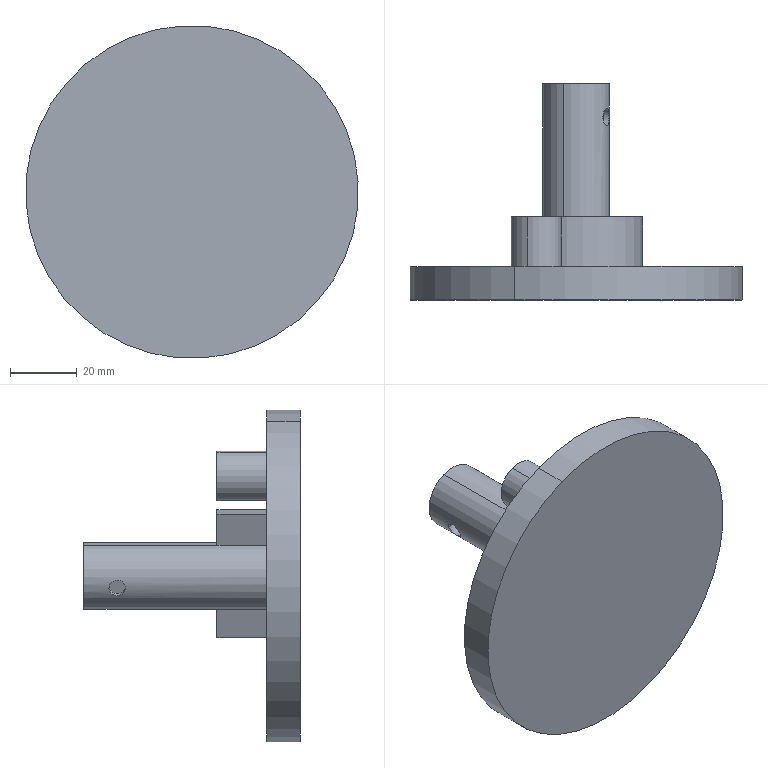Part | STEP file | Mirror 1 | 1 solid | 20 faces | box 100 x 65 x 100 mm | volume 105462 mm3 | cylinder 11 | plane 9 | commonest cylinder face diameters 5 x4 15 x2 20 x2 100 x2 40 x1
STEP:
#1=CARTESIAN_POINT('',(-1496.174,1582.764,2813.8));
#2=VERTEX_POINT('',#1);
#3=CARTESIAN_POINT('',(-1496.174,1587.764,2813.8));
#4=VERTEX_POINT('',#3);
#5=CARTESIAN_POINT('',(-1496.174,1585.264,2813.8));
#6=DIRECTION('',(0.9295,0.,0.3689));
#7=DIRECTION('',(0.,1.,0.));
#8=AXIS2_PLACEMENT_3D('',#5,#6,#7);
#9=CIRCLE('',#8,2.5);
#10=EDGE_CURVE('',#2,#4,#9,.T.);
#11=ORIENTED_EDGE('',*,*,#10,.T.);
#12=CARTESIAN_POINT('',(-1498.033,1587.764,2813.062));
#13=VERTEX_POINT('',#12);
#14=CARTESIAN_POINT('',(-1496.174,1587.764,2813.8));
#15=DIRECTION('',(0.9295,0.,0.3689));
#16=VECTOR('',#15,1000.);
#17=LINE('',#14,#16);
#18=EDGE_CURVE('',#13,#4,#17,.T.);
#19=ORIENTED_EDGE('',*,*,#18,.F.);
#20=CARTESIAN_POINT('',(-1498.033,1582.764,2813.062));
#21=VERTEX_POINT('',#20);
#22=CARTESIAN_POINT('',(-1498.033,1587.764,2813.062));
#23=CARTESIAN_POINT('',(-1497.972,1587.764,2812.908));
#24=CARTESIAN_POINT('',(-1497.908,1587.748,2812.758));
#25=CARTESIAN_POINT('',(-1497.775,1587.684,2812.466));
#26=CARTESIAN_POINT('',(-1497.706,1587.636,2812.322));
#27=CARTESIAN_POINT('',(-1497.567,1587.51,2812.052));
#28=CARTESIAN_POINT('',(-1497.498,1587.433,2811.925));
#29=CARTESIAN_POINT('',(-1497.363,1587.252,2811.687));
#30=CARTESIAN_POINT('',(-1497.296,1587.147,2811.576));
#31=CARTESIAN_POINT('',(-1497.111,1586.802,2811.279));
#32=CARTESIAN_POINT('',(-1497.004,1586.525,2811.121));
#33=CARTESIAN_POINT('',(-1496.894,1586.074,2810.963));
#34=CARTESIAN_POINT('',(-1496.865,1585.916,2810.923));
#35=CARTESIAN_POINT('',(-1496.826,1585.593,2810.869));
#36=CARTESIAN_POINT('',(-1496.816,1585.43,2810.855));
#37=CARTESIAN_POINT('',(-1496.816,1585.103,2810.855));
#38=CARTESIAN_POINT('',(-1496.826,1584.936,2810.869));
#39=CARTESIAN_POINT('',(-1496.864,1584.615,2810.922));
#40=CARTESIAN_POINT('',(-1496.893,1584.459,2810.962));
#41=CARTESIAN_POINT('',(-1497.004,1584.004,2811.121));
#42=CARTESIAN_POINT('',(-1497.11,1583.729,2811.276));
#43=CARTESIAN_POINT('',(-1497.296,1583.382,2811.576));
#44=CARTESIAN_POINT('',(-1497.361,1583.279,2811.685));
#45=CARTESIAN_POINT('',(-1497.496,1583.097,2811.922));
#46=CARTESIAN_POINT('',(-1497.567,1583.019,2812.051));
#47=CARTESIAN_POINT('',(-1497.705,1582.893,2812.321));
#48=CARTESIAN_POINT('',(-1497.773,1582.846,2812.462));
#49=CARTESIAN_POINT('',(-1497.907,1582.781,2812.755));
#50=CARTESIAN_POINT('',(-1497.972,1582.764,2812.908));
#51=CARTESIAN_POINT('',(-1498.033,1582.764,2813.062));
#52=B_SPLINE_CURVE_WITH_KNOTS('',3,(#22,#23,#24,#25,#26,#27,#28,#29,#30,#31,#32,#33,#34,#35,#36,#37,#38,#39,#40,#41,#42,#43,#44,#45,#46,#47,#48,#49,#50,#51),.UNSPECIFIED.,.F.,.F.,(4,2,2,2,2,2,2,2,2,2,2,2,2,2,4),(0.,0.0004903,0.0009806,0.001471,0.001961,0.002942,0.003432,0.003922,0.004413,0.004903,0.005884,0.006374,0.006864,0.007355,0.007845),.UNSPECIFIED.);
#53=EDGE_CURVE('',#13,#21,#52,.T.);
#54=ORIENTED_EDGE('',*,*,#53,.T.);
#55=CARTESIAN_POINT('',(-1496.174,1582.764,2813.8));
#56=DIRECTION('',(0.9295,0.,0.3689));
#57=VECTOR('',#56,1000.);
#58=LINE('',#55,#57);
#59=EDGE_CURVE('',#21,#2,#58,.T.);
#60=ORIENTED_EDGE('',*,*,#59,.T.);
#61=EDGE_LOOP('',(#11,#19,#54,#60));
#62=FACE_OUTER_BOUND('',#61,.T.);
#63=CARTESIAN_POINT('',(-1496.174,1585.264,2813.8));
#64=DIRECTION('',(-0.9295,0.,-0.3689));
#65=DIRECTION('',(0.,1.,0.));
#66=AXIS2_PLACEMENT_3D('',#63,#64,#65);
#67=CYLINDRICAL_SURFACE('',#66,2.5);
#68=ADVANCED_FACE('',(#62),#67,.F.);
#69=CARTESIAN_POINT('',(-1481.302,1582.764,2819.702));
#70=VERTEX_POINT('',#69);
#71=CARTESIAN_POINT('',(-1481.302,1587.764,2819.702));
#72=VERTEX_POINT('',#71);
#73=CARTESIAN_POINT('',(-1481.302,1585.264,2819.702));
#74=DIRECTION('',(0.9295,0.,0.3689));
#75=DIRECTION('',(0.,1.,0.));
#76=AXIS2_PLACEMENT_3D('',#73,#74,#75);
#77=CIRCLE('',#76,2.5);
#78=EDGE_CURVE('',#70,#72,#77,.T.);
#79=ORIENTED_EDGE('',*,*,#78,.F.);
#80=CARTESIAN_POINT('',(-1479.444,1582.764,2820.44));
#81=VERTEX_POINT('',#80);
#82=CARTESIAN_POINT('',(-1481.302,1582.764,2819.702));
#83=DIRECTION('',(0.9295,0.,0.3689));
#84=VECTOR('',#83,1000.);
#85=LINE('',#82,#84);
#86=EDGE_CURVE('',#70,#81,#85,.T.);
#87=ORIENTED_EDGE('',*,*,#86,.T.);
#88=CARTESIAN_POINT('',(-1479.444,1587.764,2820.44));
#89=VERTEX_POINT('',#88);
#90=CARTESIAN_POINT('',(-1479.444,1587.764,2820.44));
#91=CARTESIAN_POINT('',(-1479.382,1587.764,2820.285));
#92=CARTESIAN_POINT('',(-1479.326,1587.748,2820.132));
#93=CARTESIAN_POINT('',(-1479.222,1587.684,2819.829));
#94=CARTESIAN_POINT('',(-1479.175,1587.636,2819.677));
#95=CARTESIAN_POINT('',(-1479.09,1587.51,2819.385));
#96=CARTESIAN_POINT('',(-1479.053,1587.433,2819.245));
#97=CARTESIAN_POINT('',(-1478.989,1587.252,2818.979));
#98=CARTESIAN_POINT('',(-1478.961,1587.147,2818.853));
#99=CARTESIAN_POINT('',(-1478.891,1586.802,2818.51));
#100=CARTESIAN_POINT('',(-1478.862,1586.525,2818.321));
#101=CARTESIAN_POINT('',(-1478.834,1586.074,2818.131));
#102=CARTESIAN_POINT('',(-1478.827,1585.916,2818.081));
#103=CARTESIAN_POINT('',(-1478.819,1585.593,2818.015));
#104=CARTESIAN_POINT('',(-1478.816,1585.43,2817.999));
#105=CARTESIAN_POINT('',(-1478.816,1585.103,2817.999));
#106=CARTESIAN_POINT('',(-1478.819,1584.936,2818.015));
#107=CARTESIAN_POINT('',(-1478.827,1584.615,2818.081));
#108=CARTESIAN_POINT('',(-1478.834,1584.459,2818.129));
#109=CARTESIAN_POINT('',(-1478.861,1584.004,2818.321));
#110=CARTESIAN_POINT('',(-1478.891,1583.729,2818.507));
#111=CARTESIAN_POINT('',(-1478.961,1583.382,2818.853));
#112=CARTESIAN_POINT('',(-1478.988,1583.279,2818.977));
#113=CARTESIAN_POINT('',(-1479.053,1583.097,2819.242));
#114=CARTESIAN_POINT('',(-1479.09,1583.019,2819.384));
#115=CARTESIAN_POINT('',(-1479.174,1582.893,2819.676));
#116=CARTESIAN_POINT('',(-1479.221,1582.846,2819.825));
#117=CARTESIAN_POINT('',(-1479.325,1582.781,2820.13));
#118=CARTESIAN_POINT('',(-1479.382,1582.764,2820.285));
#119=CARTESIAN_POINT('',(-1479.444,1582.764,2820.44));
#120=B_SPLINE_CURVE_WITH_KNOTS('',3,(#90,#91,#92,#93,#94,#95,#96,#97,#98,#99,#100,#101,#102,#103,#104,#105,#106,#107,#108,#109,#110,#111,#112,#113,#114,#115,#116,#117,#118,#119),.UNSPECIFIED.,.F.,.F.,(4,2,2,2,2,2,2,2,2,2,2,2,2,2,4),(0.,0.0004903,0.0009806,0.001471,0.001961,0.002942,0.003432,0.003922,0.004413,0.004903,0.005884,0.006374,0.006864,0.007355,0.007845),.UNSPECIFIED.);
#121=EDGE_CURVE('',#89,#81,#120,.T.);
#122=ORIENTED_EDGE('',*,*,#121,.F.);
#123=CARTESIAN_POINT('',(-1481.302,1587.764,2819.702));
#124=DIRECTION('',(0.9295,0.,0.3689));
#125=VECTOR('',#124,1000.);
#126=LINE('',#123,#125);
#127=EDGE_CURVE('',#72,#89,#126,.T.);
#128=ORIENTED_EDGE('',*,*,#127,.F.);
#129=EDGE_LOOP('',(#79,#87,#122,#128));
#130=FACE_OUTER_BOUND('',#129,.T.);
#131=CARTESIAN_POINT('',(-1481.302,1585.264,2819.702));
#132=DIRECTION('',(0.9295,0.,0.3689));
#133=DIRECTION('',(0.,-1.,0.));
#134=AXIS2_PLACEMENT_3D('',#131,#132,#133);
#135=CYLINDRICAL_SURFACE('',#134,2.5);
#136=ADVANCED_FACE('',(#130),#135,.F.);
#137=CARTESIAN_POINT('',(-1503.438,1555.264,2853.79));
#138=VERTEX_POINT('',#137);
#139=CARTESIAN_POINT('',(-1497.905,1555.264,2839.848));
#140=VERTEX_POINT('',#139);
#141=CARTESIAN_POINT('',(-1500.672,1555.264,2846.819));
#142=DIRECTION('',(0.,1.,0.));
#143=DIRECTION('',(-0.3689,0.,0.9295));
#144=AXIS2_PLACEMENT_3D('',#141,#142,#143);
#145=CIRCLE('',#144,7.5);
#146=EDGE_CURVE('',#138,#140,#145,.T.);
#147=ORIENTED_EDGE('',*,*,#146,.F.);
#148=CARTESIAN_POINT('',(-1503.438,1540.264,2853.79));
#149=VERTEX_POINT('',#148);
#150=CARTESIAN_POINT('',(-1503.438,1555.264,2853.79));
#151=DIRECTION('',(0.,1.,0.));
#152=VECTOR('',#151,1000.);
#153=LINE('',#150,#152);
#154=EDGE_CURVE('',#149,#138,#153,.T.);
#155=ORIENTED_EDGE('',*,*,#154,.F.);
#156=CARTESIAN_POINT('',(-1497.905,1540.264,2839.848));
#157=VERTEX_POINT('',#156);
#158=CARTESIAN_POINT('',(-1500.672,1540.264,2846.819));
#159=DIRECTION('',(0.,1.,0.));
#160=DIRECTION('',(-0.3689,0.,0.9295));
#161=AXIS2_PLACEMENT_3D('',#158,#159,#160);
#162=CIRCLE('',#161,7.5);
#163=EDGE_CURVE('',#149,#157,#162,.T.);
#164=ORIENTED_EDGE('',*,*,#163,.T.);
#165=CARTESIAN_POINT('',(-1497.905,1555.264,2839.848));
#166=DIRECTION('',(0.,1.,0.));
#167=VECTOR('',#166,1000.);
#168=LINE('',#165,#167);
#169=EDGE_CURVE('',#157,#140,#168,.T.);
#170=ORIENTED_EDGE('',*,*,#169,.T.);
#171=EDGE_LOOP('',(#147,#155,#164,#170));
#172=FACE_OUTER_BOUND('',#171,.T.);
#173=CARTESIAN_POINT('',(-1500.672,1555.264,2846.819));
#174=DIRECTION('',(0.,-1.,0.));
#175=DIRECTION('',(-0.3689,0.,0.9295));
#176=AXIS2_PLACEMENT_3D('',#173,#174,#175);
#177=CYLINDRICAL_SURFACE('',#176,7.5);
#178=ADVANCED_FACE('',(#172),#177,.T.);
#179=CARTESIAN_POINT('',(-1507.183,1540.264,2863.224));
#180=VERTEX_POINT('',#179);
#181=CARTESIAN_POINT('',(-1470.294,1540.264,2770.277));
#182=VERTEX_POINT('',#181);
#183=CARTESIAN_POINT('',(-1488.738,1540.264,2816.751));
#184=DIRECTION('',(0.,1.,0.));
#185=DIRECTION('',(-0.3689,0.,0.9295));
#186=AXIS2_PLACEMENT_3D('',#183,#184,#185);
#187=CIRCLE('',#186,50.);
#188=EDGE_CURVE('',#180,#182,#187,.T.);
#189=ORIENTED_EDGE('',*,*,#188,.F.);
#190=CARTESIAN_POINT('',(-1507.183,1530.264,2863.224));
#191=VERTEX_POINT('',#190);
#192=CARTESIAN_POINT('',(-1507.183,1540.264,2863.224));
#193=DIRECTION('',(0.,1.,0.));
#194=VECTOR('',#193,1000.);
#195=LINE('',#192,#194);
#196=EDGE_CURVE('',#191,#180,#195,.T.);
#197=ORIENTED_EDGE('',*,*,#196,.F.);
#198=CARTESIAN_POINT('',(-1470.294,1530.264,2770.277));
#199=VERTEX_POINT('',#198);
#200=CARTESIAN_POINT('',(-1488.738,1530.264,2816.751));
#201=DIRECTION('',(0.,1.,0.));
#202=DIRECTION('',(-0.3689,0.,0.9295));
#203=AXIS2_PLACEMENT_3D('',#200,#201,#202);
#204=CIRCLE('',#203,50.);
#205=EDGE_CURVE('',#191,#199,#204,.T.);
#206=ORIENTED_EDGE('',*,*,#205,.T.);
#207=CARTESIAN_POINT('',(-1470.294,1540.264,2770.277));
#208=DIRECTION('',(0.,1.,0.));
#209=VECTOR('',#208,1000.);
#210=LINE('',#207,#209);
#211=EDGE_CURVE('',#199,#182,#210,.T.);
#212=ORIENTED_EDGE('',*,*,#211,.T.);
#213=EDGE_LOOP('',(#189,#197,#206,#212));
#214=FACE_OUTER_BOUND('',#213,.T.);
#215=CARTESIAN_POINT('',(-1488.738,1540.264,2816.751));
#216=DIRECTION('',(0.,-1.,0.));
#217=DIRECTION('',(-0.3689,0.,0.9295));
#218=AXIS2_PLACEMENT_3D('',#215,#216,#217);
#219=CYLINDRICAL_SURFACE('',#218,50.);
#220=ADVANCED_FACE('',(#214),#219,.T.);
#221=ORIENTED_EDGE('',*,*,#121,.T.);
#222=CARTESIAN_POINT('',(-1479.444,1582.764,2820.44));
#223=CARTESIAN_POINT('',(-1479.505,1582.764,2820.594));
#224=CARTESIAN_POINT('',(-1479.569,1582.781,2820.744));
#225=CARTESIAN_POINT('',(-1479.701,1582.845,2821.036));
#226=CARTESIAN_POINT('',(-1479.771,1582.893,2821.179));
#227=CARTESIAN_POINT('',(-1479.91,1583.019,2821.45));
#228=CARTESIAN_POINT('',(-1479.979,1583.095,2821.576));
#229=CARTESIAN_POINT('',(-1480.114,1583.277,2821.814));
#230=CARTESIAN_POINT('',(-1480.181,1583.382,2821.926));
#231=CARTESIAN_POINT('',(-1480.365,1583.726,2822.223));
#232=CARTESIAN_POINT('',(-1480.472,1584.004,2822.38));
#233=CARTESIAN_POINT('',(-1480.583,1584.455,2822.538));
#234=CARTESIAN_POINT('',(-1480.612,1584.613,2822.579));
#235=CARTESIAN_POINT('',(-1480.651,1584.936,2822.633));
#236=CARTESIAN_POINT('',(-1480.661,1585.098,2822.646));
#237=CARTESIAN_POINT('',(-1480.661,1585.426,2822.646));
#238=CARTESIAN_POINT('',(-1480.651,1585.592,2822.633));
#239=CARTESIAN_POINT('',(-1480.612,1585.913,2822.579));
#240=CARTESIAN_POINT('',(-1480.584,1586.069,2822.54));
#241=CARTESIAN_POINT('',(-1480.473,1586.525,2822.381));
#242=CARTESIAN_POINT('',(-1480.367,1586.8,2822.225));
#243=CARTESIAN_POINT('',(-1480.18,1587.147,2821.925));
#244=CARTESIAN_POINT('',(-1480.115,1587.25,2821.816));
#245=CARTESIAN_POINT('',(-1479.98,1587.431,2821.579));
#246=CARTESIAN_POINT('',(-1479.91,1587.51,2821.45));
#247=CARTESIAN_POINT('',(-1479.772,1587.635,2821.18));
#248=CARTESIAN_POINT('',(-1479.703,1587.683,2821.04));
#249=CARTESIAN_POINT('',(-1479.57,1587.748,2820.746));
#250=CARTESIAN_POINT('',(-1479.505,1587.764,2820.594));
#251=CARTESIAN_POINT('',(-1479.444,1587.764,2820.44));
#252=B_SPLINE_CURVE_WITH_KNOTS('',3,(#222,#223,#224,#225,#226,#227,#228,#229,#230,#231,#232,#233,#234,#235,#236,#237,#238,#239,#240,#241,#242,#243,#244,#245,#246,#247,#248,#249,#250,#251),.UNSPECIFIED.,.F.,.F.,(4,2,2,2,2,2,2,2,2,2,2,2,2,2,4),(0.,0.0004903,0.0009806,0.001471,0.001961,0.002942,0.003432,0.003922,0.004413,0.004903,0.005884,0.006374,0.006864,0.007355,0.007845),.UNSPECIFIED.);
#253=EDGE_CURVE('',#81,#89,#252,.T.);
#254=ORIENTED_EDGE('',*,*,#253,.T.);
#255=EDGE_LOOP('',(#221,#254));
#256=FACE_BOUND('',#255,.T.);
#257=CARTESIAN_POINT('',(-1492.427,1595.264,2826.045));
#258=VERTEX_POINT('',#257);
#259=CARTESIAN_POINT('',(-1485.049,1595.264,2807.456));
#260=VERTEX_POINT('',#259);
#261=CARTESIAN_POINT('',(-1488.738,1595.264,2816.751));
#262=DIRECTION('',(0.,1.,0.));
#263=DIRECTION('',(-0.3689,0.,0.9295));
#264=AXIS2_PLACEMENT_3D('',#261,#262,#263);
#265=CIRCLE('',#264,10.);
#266=EDGE_CURVE('',#258,#260,#265,.T.);
#267=ORIENTED_EDGE('',*,*,#266,.F.);
#268=CARTESIAN_POINT('',(-1492.427,1555.264,2826.045));
#269=VERTEX_POINT('',#268);
#270=CARTESIAN_POINT('',(-1492.427,1595.264,2826.045));
#271=DIRECTION('',(0.,1.,0.));
#272=VECTOR('',#271,1000.);
#273=LINE('',#270,#272);
#274=EDGE_CURVE('',#269,#258,#273,.T.);
#275=ORIENTED_EDGE('',*,*,#274,.F.);
#276=CARTESIAN_POINT('',(-1485.049,1555.264,2807.456));
#277=VERTEX_POINT('',#276);
#278=CARTESIAN_POINT('',(-1488.738,1555.264,2816.751));
#279=DIRECTION('',(0.,1.,0.));
#280=DIRECTION('',(-0.3689,0.,0.9295));
#281=AXIS2_PLACEMENT_3D('',#278,#279,#280);
#282=CIRCLE('',#281,10.);
#283=EDGE_CURVE('',#269,#277,#282,.T.);
#284=ORIENTED_EDGE('',*,*,#283,.T.);
#285=CARTESIAN_POINT('',(-1485.049,1595.264,2807.456));
#286=DIRECTION('',(0.,1.,0.));
#287=VECTOR('',#286,1000.);
#288=LINE('',#285,#287);
#289=EDGE_CURVE('',#277,#260,#288,.T.);
#290=ORIENTED_EDGE('',*,*,#289,.T.);
#291=EDGE_LOOP('',(#267,#275,#284,#290));
#292=FACE_OUTER_BOUND('',#291,.T.);
#293=CARTESIAN_POINT('',(-1488.738,1595.264,2816.751));
#294=DIRECTION('',(0.,-1.,0.));
#295=DIRECTION('',(-0.3689,0.,0.9295));
#296=AXIS2_PLACEMENT_3D('',#293,#294,#295);
#297=CYLINDRICAL_SURFACE('',#296,10.);
#298=ADVANCED_FACE('',(#256,#292),#297,.T.);
#299=ORIENTED_EDGE('',*,*,#274,.T.);
#300=CARTESIAN_POINT('',(-1488.738,1595.264,2816.751));
#301=DIRECTION('',(0.,1.,0.));
#302=DIRECTION('',(-0.3689,0.,0.9295));
#303=AXIS2_PLACEMENT_3D('',#300,#301,#302);
#304=CIRCLE('',#303,10.);
#305=EDGE_CURVE('',#260,#258,#304,.T.);
#306=ORIENTED_EDGE('',*,*,#305,.F.);
#307=ORIENTED_EDGE('',*,*,#289,.F.);
#308=CARTESIAN_POINT('',(-1485.049,1540.264,2807.456));
#309=VERTEX_POINT('',#308);
#310=CARTESIAN_POINT('',(-1485.049,1511.98,2807.456));
#311=DIRECTION('',(0.,-1.,0.));
#312=VECTOR('',#311,1000.);
#313=LINE('',#310,#312);
#314=EDGE_CURVE('',#277,#309,#313,.T.);
#315=ORIENTED_EDGE('',*,*,#314,.T.);
#316=CARTESIAN_POINT('',(-1492.427,1540.264,2826.045));
#317=VERTEX_POINT('',#316);
#318=CARTESIAN_POINT('',(-1488.738,1540.264,2816.751));
#319=DIRECTION('',(0.,1.,0.));
#320=DIRECTION('',(-0.3689,0.,0.9295));
#321=AXIS2_PLACEMENT_3D('',#318,#319,#320);
#322=CIRCLE('',#321,10.);
#323=EDGE_CURVE('',#309,#317,#322,.T.);
#324=ORIENTED_EDGE('',*,*,#323,.T.);
#325=CARTESIAN_POINT('',(-1492.427,1511.98,2826.045));
#326=DIRECTION('',(0.,1.,0.));
#327=VECTOR('',#326,1000.);
#328=LINE('',#325,#327);
#329=EDGE_CURVE('',#317,#269,#328,.T.);
#330=ORIENTED_EDGE('',*,*,#329,.T.);
#331=EDGE_LOOP('',(#299,#306,#307,#315,#324,#330));
#332=FACE_OUTER_BOUND('',#331,.T.);
#333=CARTESIAN_POINT('',(-1498.033,1582.764,2813.062));
#334=CARTESIAN_POINT('',(-1498.094,1582.764,2813.216));
#335=CARTESIAN_POINT('',(-1498.15,1582.781,2813.369));
#336=CARTESIAN_POINT('',(-1498.254,1582.845,2813.672));
#337=CARTESIAN_POINT('',(-1498.302,1582.893,2813.825));
#338=CARTESIAN_POINT('',(-1498.386,1583.019,2814.117));
#339=CARTESIAN_POINT('',(-1498.423,1583.095,2814.256));
#340=CARTESIAN_POINT('',(-1498.488,1583.277,2814.522));
#341=CARTESIAN_POINT('',(-1498.516,1583.382,2814.649));
#342=CARTESIAN_POINT('',(-1498.585,1583.726,2814.992));
#343=CARTESIAN_POINT('',(-1498.615,1584.004,2815.18));
#344=CARTESIAN_POINT('',(-1498.643,1584.455,2815.371));
#345=CARTESIAN_POINT('',(-1498.649,1584.613,2815.42));
#346=CARTESIAN_POINT('',(-1498.658,1584.936,2815.486));
#347=CARTESIAN_POINT('',(-1498.66,1585.098,2815.502));
#348=CARTESIAN_POINT('',(-1498.66,1585.426,2815.503));
#349=CARTESIAN_POINT('',(-1498.658,1585.592,2815.486));
#350=CARTESIAN_POINT('',(-1498.649,1585.913,2815.421));
#351=CARTESIAN_POINT('',(-1498.643,1586.069,2815.372));
#352=CARTESIAN_POINT('',(-1498.615,1586.525,2815.18));
#353=CARTESIAN_POINT('',(-1498.586,1586.8,2814.994));
#354=CARTESIAN_POINT('',(-1498.516,1587.147,2814.649));
#355=CARTESIAN_POINT('',(-1498.488,1587.25,2814.525));
#356=CARTESIAN_POINT('',(-1498.424,1587.431,2814.26));
#357=CARTESIAN_POINT('',(-1498.386,1587.51,2814.117));
#358=CARTESIAN_POINT('',(-1498.302,1587.635,2813.826));
#359=CARTESIAN_POINT('',(-1498.255,1587.683,2813.677));
#360=CARTESIAN_POINT('',(-1498.152,1587.748,2813.372));
#361=CARTESIAN_POINT('',(-1498.094,1587.764,2813.216));
#362=CARTESIAN_POINT('',(-1498.033,1587.764,2813.062));
#363=B_SPLINE_CURVE_WITH_KNOTS('',3,(#333,#334,#335,#336,#337,#338,#339,#340,#341,#342,#343,#344,#345,#346,#347,#348,#349,#350,#351,#352,#353,#354,#355,#356,#357,#358,#359,#360,#361,#362),.UNSPECIFIED.,.F.,.F.,(4,2,2,2,2,2,2,2,2,2,2,2,2,2,4),(0.,0.0004903,0.0009806,0.001471,0.001961,0.002942,0.003432,0.003922,0.004413,0.004903,0.005884,0.006374,0.006864,0.007355,0.007845),.UNSPECIFIED.);
#364=EDGE_CURVE('',#21,#13,#363,.T.);
#365=ORIENTED_EDGE('',*,*,#364,.F.);
#366=ORIENTED_EDGE('',*,*,#53,.F.);
#367=EDGE_LOOP('',(#365,#366));
#368=FACE_BOUND('',#367,.T.);
#369=CARTESIAN_POINT('',(-1488.738,1595.264,2816.751));
#370=DIRECTION('',(0.,-1.,0.));
#371=DIRECTION('',(-0.3689,0.,0.9295));
#372=AXIS2_PLACEMENT_3D('',#369,#370,#371);
#373=CYLINDRICAL_SURFACE('',#372,10.);
#374=ADVANCED_FACE('',(#332,#368),#373,.T.);
#375=CARTESIAN_POINT('',(-1500.672,1540.264,2846.819));
#376=DIRECTION('',(0.,1.,0.));
#377=DIRECTION('',(-0.3689,0.,0.9295));
#378=AXIS2_PLACEMENT_3D('',#375,#376,#377);
#379=CIRCLE('',#378,7.5);
#380=EDGE_CURVE('',#157,#149,#379,.T.);
#381=ORIENTED_EDGE('',*,*,#380,.F.);
#382=ORIENTED_EDGE('',*,*,#163,.F.);
#383=EDGE_LOOP('',(#381,#382));
#384=FACE_BOUND('',#383,.T.);
#385=CARTESIAN_POINT('',(-1488.738,1540.264,2816.751));
#386=DIRECTION('',(0.,1.,0.));
#387=DIRECTION('',(-0.3689,0.,0.9295));
#388=AXIS2_PLACEMENT_3D('',#385,#386,#387);
#389=CIRCLE('',#388,50.);
#390=EDGE_CURVE('',#182,#180,#389,.T.);
#391=ORIENTED_EDGE('',*,*,#390,.T.);
#392=ORIENTED_EDGE('',*,*,#188,.T.);
#393=EDGE_LOOP('',(#391,#392));
#394=FACE_OUTER_BOUND('',#393,.T.);
#395=CARTESIAN_POINT('',(-1496.116,1540.264,2835.34));
#396=VERTEX_POINT('',#395);
#397=CARTESIAN_POINT('',(-1481.36,1540.264,2798.161));
#398=DIRECTION('',(-0.3689,0.,0.9295));
#399=VECTOR('',#398,1000.);
#400=LINE('',#397,#399);
#401=EDGE_CURVE('',#317,#396,#400,.T.);
#402=ORIENTED_EDGE('',*,*,#401,.F.);
#403=ORIENTED_EDGE('',*,*,#323,.F.);
#404=CARTESIAN_POINT('',(-1481.36,1540.264,2798.161));
#405=VERTEX_POINT('',#404);
#406=CARTESIAN_POINT('',(-1481.36,1540.264,2798.161));
#407=DIRECTION('',(-0.3689,0.,0.9295));
#408=VECTOR('',#407,1000.);
#409=LINE('',#406,#408);
#410=EDGE_CURVE('',#405,#309,#409,.T.);
#411=ORIENTED_EDGE('',*,*,#410,.F.);
#412=CARTESIAN_POINT('',(-1488.738,1540.264,2816.751));
#413=DIRECTION('',(0.,1.,0.));
#414=DIRECTION('',(-0.3689,0.,0.9295));
#415=AXIS2_PLACEMENT_3D('',#412,#413,#414);
#416=CIRCLE('',#415,20.);
#417=EDGE_CURVE('',#396,#405,#416,.T.);
#418=ORIENTED_EDGE('',*,*,#417,.F.);
#419=EDGE_LOOP('',(#402,#403,#411,#418));
#420=FACE_BOUND('',#419,.T.);
#421=CARTESIAN_POINT('',(-1488.738,1540.264,2816.751));
#422=DIRECTION('',(0.,1.,0.));
#423=DIRECTION('',(0.3689,0.,-0.9295));
#424=AXIS2_PLACEMENT_3D('',#421,#422,#423);
#425=PLANE('',#424);
#426=ADVANCED_FACE('',(#384,#394,#420),#425,.T.);
#427=ORIENTED_EDGE('',*,*,#196,.T.);
#428=ORIENTED_EDGE('',*,*,#390,.F.);
#429=ORIENTED_EDGE('',*,*,#211,.F.);
#430=CARTESIAN_POINT('',(-1488.738,1530.264,2816.751));
#431=DIRECTION('',(0.,1.,0.));
#432=DIRECTION('',(-0.3689,0.,0.9295));
#433=AXIS2_PLACEMENT_3D('',#430,#431,#432);
#434=CIRCLE('',#433,50.);
#435=EDGE_CURVE('',#199,#191,#434,.T.);
#436=ORIENTED_EDGE('',*,*,#435,.T.);
#437=EDGE_LOOP('',(#427,#428,#429,#436));
#438=FACE_OUTER_BOUND('',#437,.T.);
#439=CARTESIAN_POINT('',(-1488.738,1540.264,2816.751));
#440=DIRECTION('',(0.,-1.,0.));
#441=DIRECTION('',(-0.3689,0.,0.9295));
#442=AXIS2_PLACEMENT_3D('',#439,#440,#441);
#443=CYLINDRICAL_SURFACE('',#442,50.);
#444=ADVANCED_FACE('',(#438),#443,.T.);
#445=ORIENTED_EDGE('',*,*,#435,.F.);
#446=ORIENTED_EDGE('',*,*,#205,.F.);
#447=EDGE_LOOP('',(#445,#446));
#448=FACE_OUTER_BOUND('',#447,.T.);
#449=CARTESIAN_POINT('',(-1488.738,1530.264,2816.751));
#450=DIRECTION('',(0.,1.,0.));
#451=DIRECTION('',(0.3689,0.,-0.9295));
#452=AXIS2_PLACEMENT_3D('',#449,#450,#451);
#453=PLANE('',#452);
#454=ADVANCED_FACE('',(#448),#453,.F.);
#455=CARTESIAN_POINT('',(-1496.116,1555.264,2835.34));
#456=VERTEX_POINT('',#455);
#457=CARTESIAN_POINT('',(-1481.36,1555.264,2798.161));
#458=VERTEX_POINT('',#457);
#459=CARTESIAN_POINT('',(-1488.738,1555.264,2816.751));
#460=DIRECTION('',(0.,1.,0.));
#461=DIRECTION('',(-0.3689,0.,0.9295));
#462=AXIS2_PLACEMENT_3D('',#459,#460,#461);
#463=CIRCLE('',#462,20.);
#464=EDGE_CURVE('',#456,#458,#463,.T.);
#465=ORIENTED_EDGE('',*,*,#464,.F.);
#466=CARTESIAN_POINT('',(-1496.116,1495.543,2835.34));
#467=DIRECTION('',(0.,1.,0.));
#468=VECTOR('',#467,1000.);
#469=LINE('',#466,#468);
#470=EDGE_CURVE('',#396,#456,#469,.T.);
#471=ORIENTED_EDGE('',*,*,#470,.F.);
#472=ORIENTED_EDGE('',*,*,#417,.T.);
#473=CARTESIAN_POINT('',(-1481.36,1495.543,2798.161));
#474=DIRECTION('',(0.,1.,0.));
#475=VECTOR('',#474,1000.);
#476=LINE('',#473,#475);
#477=EDGE_CURVE('',#405,#458,#476,.T.);
#478=ORIENTED_EDGE('',*,*,#477,.T.);
#479=EDGE_LOOP('',(#465,#471,#472,#478));
#480=FACE_OUTER_BOUND('',#479,.T.);
#481=CARTESIAN_POINT('',(-1488.738,1555.264,2816.751));
#482=DIRECTION('',(0.,-1.,0.));
#483=DIRECTION('',(-0.3689,0.,0.9295));
#484=AXIS2_PLACEMENT_3D('',#481,#482,#483);
#485=CYLINDRICAL_SURFACE('',#484,20.);
#486=ADVANCED_FACE('',(#480),#485,.T.);
#487=CARTESIAN_POINT('',(-1481.36,1555.264,2798.161));
#488=DIRECTION('',(0.3689,0.,-0.9295));
#489=VECTOR('',#488,1000.);
#490=LINE('',#487,#489);
#491=EDGE_CURVE('',#456,#269,#490,.T.);
#492=ORIENTED_EDGE('',*,*,#491,.F.);
#493=ORIENTED_EDGE('',*,*,#464,.T.);
#494=CARTESIAN_POINT('',(-1481.36,1555.264,2798.161));
#495=DIRECTION('',(0.3689,0.,-0.9295));
#496=VECTOR('',#495,1000.);
#497=LINE('',#494,#496);
#498=EDGE_CURVE('',#277,#458,#497,.T.);
#499=ORIENTED_EDGE('',*,*,#498,.F.);
#500=ORIENTED_EDGE('',*,*,#283,.F.);
#501=EDGE_LOOP('',(#492,#493,#499,#500));
#502=FACE_OUTER_BOUND('',#501,.T.);
#503=CARTESIAN_POINT('',(-1488.738,1555.264,2816.751));
#504=DIRECTION('',(0.,1.,0.));
#505=DIRECTION('',(0.3689,0.,-0.9295));
#506=AXIS2_PLACEMENT_3D('',#503,#504,#505);
#507=PLANE('',#506);
#508=ADVANCED_FACE('',(#502),#507,.T.);
#509=ORIENTED_EDGE('',*,*,#154,.T.);
#510=CARTESIAN_POINT('',(-1500.672,1555.264,2846.819));
#511=DIRECTION('',(0.,1.,0.));
#512=DIRECTION('',(-0.3689,0.,0.9295));
#513=AXIS2_PLACEMENT_3D('',#510,#511,#512);
#514=CIRCLE('',#513,7.5);
#515=EDGE_CURVE('',#140,#138,#514,.T.);
#516=ORIENTED_EDGE('',*,*,#515,.F.);
#517=ORIENTED_EDGE('',*,*,#169,.F.);
#518=ORIENTED_EDGE('',*,*,#380,.T.);
#519=EDGE_LOOP('',(#509,#516,#517,#518));
#520=FACE_OUTER_BOUND('',#519,.T.);
#521=CARTESIAN_POINT('',(-1500.672,1555.264,2846.819));
#522=DIRECTION('',(0.,-1.,0.));
#523=DIRECTION('',(-0.3689,0.,0.9295));
#524=AXIS2_PLACEMENT_3D('',#521,#522,#523);
#525=CYLINDRICAL_SURFACE('',#524,7.5);
#526=ADVANCED_FACE('',(#520),#525,.T.);
#527=ORIENTED_EDGE('',*,*,#515,.T.);
#528=ORIENTED_EDGE('',*,*,#146,.T.);
#529=EDGE_LOOP('',(#527,#528));
#530=FACE_OUTER_BOUND('',#529,.T.);
#531=CARTESIAN_POINT('',(-1500.672,1555.264,2846.819));
#532=DIRECTION('',(0.,1.,0.));
#533=DIRECTION('',(0.3689,0.,-0.9295));
#534=AXIS2_PLACEMENT_3D('',#531,#532,#533);
#535=PLANE('',#534);
#536=ADVANCED_FACE('',(#530),#535,.T.);
#537=ORIENTED_EDGE('',*,*,#498,.T.);
#538=ORIENTED_EDGE('',*,*,#477,.F.);
#539=ORIENTED_EDGE('',*,*,#410,.T.);
#540=ORIENTED_EDGE('',*,*,#314,.F.);
#541=EDGE_LOOP('',(#537,#538,#539,#540));
#542=FACE_OUTER_BOUND('',#541,.T.);
#543=CARTESIAN_POINT('',(-1481.36,1495.543,2798.161));
#544=DIRECTION('',(0.9295,0.,0.3689));
#545=DIRECTION('',(0.,-1.,0.));
#546=AXIS2_PLACEMENT_3D('',#543,#544,#545);
#547=PLANE('',#546);
#548=ADVANCED_FACE('',(#542),#547,.F.);
#549=ORIENTED_EDGE('',*,*,#401,.T.);
#550=ORIENTED_EDGE('',*,*,#470,.T.);
#551=ORIENTED_EDGE('',*,*,#491,.T.);
#552=ORIENTED_EDGE('',*,*,#329,.F.);
#553=EDGE_LOOP('',(#549,#550,#551,#552));
#554=FACE_OUTER_BOUND('',#553,.T.);
#555=CARTESIAN_POINT('',(-1481.36,1495.543,2798.161));
#556=DIRECTION('',(0.9295,0.,0.3689));
#557=DIRECTION('',(0.,-1.,0.));
#558=AXIS2_PLACEMENT_3D('',#555,#556,#557);
#559=PLANE('',#558);
#560=ADVANCED_FACE('',(#554),#559,.F.);
#561=ORIENTED_EDGE('',*,*,#305,.T.);
#562=ORIENTED_EDGE('',*,*,#266,.T.);
#563=EDGE_LOOP('',(#561,#562));
#564=FACE_OUTER_BOUND('',#563,.T.);
#565=CARTESIAN_POINT('',(-1488.738,1595.264,2816.751));
#566=DIRECTION('',(0.,1.,0.));
#567=DIRECTION('',(0.3689,0.,-0.9295));
#568=AXIS2_PLACEMENT_3D('',#565,#566,#567);
#569=PLANE('',#568);
#570=ADVANCED_FACE('',(#564),#569,.T.);
#571=ORIENTED_EDGE('',*,*,#86,.F.);
#572=CARTESIAN_POINT('',(-1481.302,1585.264,2819.702));
#573=DIRECTION('',(0.9295,0.,0.3689));
#574=DIRECTION('',(0.,1.,0.));
#575=AXIS2_PLACEMENT_3D('',#572,#573,#574);
#576=CIRCLE('',#575,2.5);
#577=EDGE_CURVE('',#72,#70,#576,.T.);
#578=ORIENTED_EDGE('',*,*,#577,.F.);
#579=ORIENTED_EDGE('',*,*,#127,.T.);
#580=ORIENTED_EDGE('',*,*,#253,.F.);
#581=EDGE_LOOP('',(#571,#578,#579,#580));
#582=FACE_OUTER_BOUND('',#581,.T.);
#583=CARTESIAN_POINT('',(-1481.302,1585.264,2819.702));
#584=DIRECTION('',(0.9295,0.,0.3689));
#585=DIRECTION('',(0.,-1.,0.));
#586=AXIS2_PLACEMENT_3D('',#583,#584,#585);
#587=CYLINDRICAL_SURFACE('',#586,2.5);
#588=ADVANCED_FACE('',(#582),#587,.F.);
#589=ORIENTED_EDGE('',*,*,#577,.T.);
#590=ORIENTED_EDGE('',*,*,#78,.T.);
#591=EDGE_LOOP('',(#589,#590));
#592=FACE_OUTER_BOUND('',#591,.T.);
#593=CARTESIAN_POINT('',(-1481.302,1585.264,2819.702));
#594=DIRECTION('',(0.9295,0.,0.3689));
#595=DIRECTION('',(0.,-1.,0.));
#596=AXIS2_PLACEMENT_3D('',#593,#594,#595);
#597=PLANE('',#596);
#598=ADVANCED_FACE('',(#592),#597,.T.);
#599=ORIENTED_EDGE('',*,*,#18,.T.);
#600=CARTESIAN_POINT('',(-1496.174,1585.264,2813.8));
#601=DIRECTION('',(0.9295,0.,0.3689));
#602=DIRECTION('',(0.,1.,0.));
#603=AXIS2_PLACEMENT_3D('',#600,#601,#602);
#604=CIRCLE('',#603,2.5);
#605=EDGE_CURVE('',#4,#2,#604,.T.);
#606=ORIENTED_EDGE('',*,*,#605,.T.);
#607=ORIENTED_EDGE('',*,*,#59,.F.);
#608=ORIENTED_EDGE('',*,*,#364,.T.);
#609=EDGE_LOOP('',(#599,#606,#607,#608));
#610=FACE_OUTER_BOUND('',#609,.T.);
#611=CARTESIAN_POINT('',(-1496.174,1585.264,2813.8));
#612=DIRECTION('',(-0.9295,0.,-0.3689));
#613=DIRECTION('',(0.,1.,0.));
#614=AXIS2_PLACEMENT_3D('',#611,#612,#613);
#615=CYLINDRICAL_SURFACE('',#614,2.5);
#616=ADVANCED_FACE('',(#610),#615,.F.);
#617=ORIENTED_EDGE('',*,*,#10,.F.);
#618=ORIENTED_EDGE('',*,*,#605,.F.);
#619=EDGE_LOOP('',(#617,#618));
#620=FACE_OUTER_BOUND('',#619,.T.);
#621=CARTESIAN_POINT('',(-1496.174,1585.264,2813.8));
#622=DIRECTION('',(-0.9295,0.,-0.3689));
#623=DIRECTION('',(0.,-1.,0.));
#624=AXIS2_PLACEMENT_3D('',#621,#622,#623);
#625=PLANE('',#624);
#626=ADVANCED_FACE('',(#620),#625,.T.);
#627=CLOSED_SHELL('',(#68,#136,#178,#220,#298,#374,#426,#444,#454,#486,#508,#526,#536,#548,#560,#570,#588,#598,#616,#626));
#628=MANIFOLD_SOLID_BREP('',#627);
#629=CARTESIAN_POINT('',(0.,0.,0.));
#630=DIRECTION('',(0.,0.,1.));
#631=DIRECTION('',(1.,0.,0.));
#632=AXIS2_PLACEMENT_3D('',#629,#630,#631);
#633=(LENGTH_UNIT()NAMED_UNIT(*)SI_UNIT(.MILLI.,.METRE.));
#634=UNCERTAINTY_MEASURE_WITH_UNIT(LENGTH_MEASURE(0.00001),#633,'','');
#635=(NAMED_UNIT(*)PLANE_ANGLE_UNIT()SI_UNIT($,.RADIAN.));
#636=(NAMED_UNIT(*)SI_UNIT($,.STERADIAN.)SOLID_ANGLE_UNIT());
#637=(GEOMETRIC_REPRESENTATION_CONTEXT(3)GLOBAL_UNCERTAINTY_ASSIGNED_CONTEXT((#634))GLOBAL_UNIT_ASSIGNED_CONTEXT((#633,#635,#636))REPRESENTATION_CONTEXT('',''));
#638=ADVANCED_BREP_SHAPE_REPRESENTATION('',(#628,#632),#637);